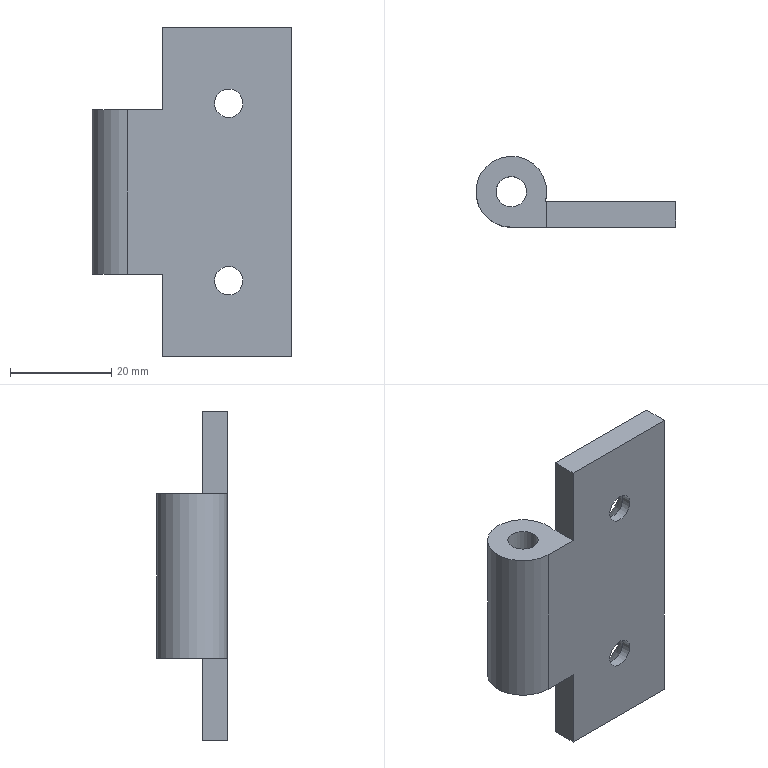Part | NX | 1 solid | 15 faces | box 39.5 x 14 x 65 mm | volume 12285 mm3 | plane 9 | cylinder 4 | cone 2 | commonest cylinder face diameters 5.6 x2 6 x1 14 x1
STEP:
#1=CARTESIAN_POINT('',(7.,0.,0.));
#2=VERTEX_POINT('',#1);
#3=CARTESIAN_POINT('',(7.,5.,0.));
#4=VERTEX_POINT('',#3);
#5=CARTESIAN_POINT('',(7.,-65.,0.));
#6=DIRECTION('',(0.,1.,0.));
#7=VECTOR('',#6,1000.);
#8=LINE('',#5,#7);
#9=EDGE_CURVE('',#2,#4,#8,.T.);
#10=ORIENTED_EDGE('',*,*,#9,.F.);
#11=CARTESIAN_POINT('',(32.5,0.,0.));
#12=VERTEX_POINT('',#11);
#13=CARTESIAN_POINT('',(0.,0.,0.));
#14=DIRECTION('',(1.,0.,0.));
#15=VECTOR('',#14,1000.);
#16=LINE('',#13,#15);
#17=EDGE_CURVE('',#2,#12,#16,.T.);
#18=ORIENTED_EDGE('',*,*,#17,.T.);
#19=CARTESIAN_POINT('',(32.5,5.,0.));
#20=VERTEX_POINT('',#19);
#21=CARTESIAN_POINT('',(32.5,0.,0.));
#22=DIRECTION('',(0.,1.,0.));
#23=VECTOR('',#22,1000.);
#24=LINE('',#21,#23);
#25=EDGE_CURVE('',#12,#20,#24,.T.);
#26=ORIENTED_EDGE('',*,*,#25,.T.);
#27=CARTESIAN_POINT('',(32.5,5.,0.));
#28=DIRECTION('',(-1.,0.,0.));
#29=VECTOR('',#28,1000.);
#30=LINE('',#27,#29);
#31=EDGE_CURVE('',#20,#4,#30,.T.);
#32=ORIENTED_EDGE('',*,*,#31,.T.);
#33=EDGE_LOOP('',(#10,#18,#26,#32));
#34=FACE_BOUND('',#33,.T.);
#35=CARTESIAN_POINT('',(0.,7.,0.));
#36=DIRECTION('',(0.,0.,1.));
#37=DIRECTION('',(1.,0.,0.));
#38=AXIS2_PLACEMENT_3D('',#35,#36,#37);
#39=PLANE('',#38);
#40=ADVANCED_FACE('',(#34),#39,.T.);
#41=CARTESIAN_POINT('',(7.,0.,-65.));
#42=VERTEX_POINT('',#41);
#43=CARTESIAN_POINT('',(32.5,0.,-65.));
#44=VERTEX_POINT('',#43);
#45=CARTESIAN_POINT('',(0.,0.,-65.));
#46=DIRECTION('',(1.,0.,0.));
#47=VECTOR('',#46,1000.);
#48=LINE('',#45,#47);
#49=EDGE_CURVE('',#42,#44,#48,.T.);
#50=ORIENTED_EDGE('',*,*,#49,.F.);
#51=CARTESIAN_POINT('',(7.,5.,-65.));
#52=VERTEX_POINT('',#51);
#53=CARTESIAN_POINT('',(7.,-65.,-65.));
#54=DIRECTION('',(0.,1.,0.));
#55=VECTOR('',#54,1000.);
#56=LINE('',#53,#55);
#57=EDGE_CURVE('',#42,#52,#56,.T.);
#58=ORIENTED_EDGE('',*,*,#57,.T.);
#59=CARTESIAN_POINT('',(32.5,5.,-65.));
#60=VERTEX_POINT('',#59);
#61=CARTESIAN_POINT('',(32.5,5.,-65.));
#62=DIRECTION('',(-1.,0.,0.));
#63=VECTOR('',#62,1000.);
#64=LINE('',#61,#63);
#65=EDGE_CURVE('',#60,#52,#64,.T.);
#66=ORIENTED_EDGE('',*,*,#65,.F.);
#67=CARTESIAN_POINT('',(32.5,0.,-65.));
#68=DIRECTION('',(0.,1.,0.));
#69=VECTOR('',#68,1000.);
#70=LINE('',#67,#69);
#71=EDGE_CURVE('',#44,#60,#70,.T.);
#72=ORIENTED_EDGE('',*,*,#71,.F.);
#73=EDGE_LOOP('',(#50,#58,#66,#72));
#74=FACE_BOUND('',#73,.T.);
#75=CARTESIAN_POINT('',(0.,7.,-65.));
#76=DIRECTION('',(0.,0.,1.));
#77=DIRECTION('',(1.,0.,0.));
#78=AXIS2_PLACEMENT_3D('',#75,#76,#77);
#79=PLANE('',#78);
#80=ADVANCED_FACE('',(#74),#79,.F.);
#81=CARTESIAN_POINT('',(0.,0.,-16.25));
#82=VERTEX_POINT('',#81);
#83=CARTESIAN_POINT('',(6.708,5.,-16.25));
#84=VERTEX_POINT('',#83);
#85=CARTESIAN_POINT('',(0.,7.,-16.25));
#86=DIRECTION('',(0.,0.,-1.));
#87=DIRECTION('',(-1.,0.,0.));
#88=AXIS2_PLACEMENT_3D('',#85,#86,#87);
#89=CIRCLE('',#88,7.);
#90=EDGE_CURVE('',#82,#84,#89,.T.);
#91=ORIENTED_EDGE('',*,*,#90,.T.);
#92=CARTESIAN_POINT('',(6.708,5.,-48.75));
#93=VERTEX_POINT('',#92);
#94=CARTESIAN_POINT('',(6.708,5.,0.));
#95=DIRECTION('',(0.,0.,-1.));
#96=VECTOR('',#95,1000.);
#97=LINE('',#94,#96);
#98=EDGE_CURVE('',#84,#93,#97,.T.);
#99=ORIENTED_EDGE('',*,*,#98,.T.);
#100=CARTESIAN_POINT('',(0.,0.,-48.75));
#101=VERTEX_POINT('',#100);
#102=CARTESIAN_POINT('',(0.,7.,-48.75));
#103=DIRECTION('',(0.,0.,1.));
#104=DIRECTION('',(1.,0.,0.));
#105=AXIS2_PLACEMENT_3D('',#102,#103,#104);
#106=CIRCLE('',#105,7.);
#107=EDGE_CURVE('',#93,#101,#106,.T.);
#108=ORIENTED_EDGE('',*,*,#107,.T.);
#109=CARTESIAN_POINT('',(0.,0.,0.));
#110=DIRECTION('',(0.,0.,-1.));
#111=VECTOR('',#110,1000.);
#112=LINE('',#109,#111);
#113=EDGE_CURVE('',#82,#101,#112,.T.);
#114=ORIENTED_EDGE('',*,*,#113,.F.);
#115=EDGE_LOOP('',(#91,#99,#108,#114));
#116=FACE_BOUND('',#115,.T.);
#117=CARTESIAN_POINT('',(0.,7.,0.));
#118=DIRECTION('',(0.,0.,-1.));
#119=DIRECTION('',(-1.,0.,0.));
#120=AXIS2_PLACEMENT_3D('',#117,#118,#119);
#121=CYLINDRICAL_SURFACE('',#120,7.);
#122=ADVANCED_FACE('',(#116),#121,.T.);
#123=CARTESIAN_POINT('',(20.,0.,-47.2));
#124=VERTEX_POINT('',#123);
#125=CARTESIAN_POINT('',(20.,0.,-50.));
#126=DIRECTION('',(0.,1.,0.));
#127=DIRECTION('',(0.,0.,1.));
#128=AXIS2_PLACEMENT_3D('',#125,#126,#127);
#129=CIRCLE('',#128,2.8);
#130=EDGE_CURVE('',#124,#124,#129,.T.);
#131=ORIENTED_EDGE('',*,*,#130,.T.);
#132=EDGE_LOOP('',(#131));
#133=FACE_BOUND('',#132,.T.);
#134=CARTESIAN_POINT('',(20.,0.,-12.2));
#135=VERTEX_POINT('',#134);
#136=CARTESIAN_POINT('',(20.,0.,-15.));
#137=DIRECTION('',(0.,1.,0.));
#138=DIRECTION('',(0.,0.,1.));
#139=AXIS2_PLACEMENT_3D('',#136,#137,#138);
#140=CIRCLE('',#139,2.8);
#141=EDGE_CURVE('',#135,#135,#140,.T.);
#142=ORIENTED_EDGE('',*,*,#141,.T.);
#143=EDGE_LOOP('',(#142));
#144=FACE_BOUND('',#143,.T.);
#145=CARTESIAN_POINT('',(7.,0.,-48.75));
#146=VERTEX_POINT('',#145);
#147=CARTESIAN_POINT('',(0.,0.,-48.75));
#148=DIRECTION('',(1.,0.,0.));
#149=VECTOR('',#148,1000.);
#150=LINE('',#147,#149);
#151=EDGE_CURVE('',#101,#146,#150,.T.);
#152=ORIENTED_EDGE('',*,*,#151,.T.);
#153=CARTESIAN_POINT('',(7.,0.,0.));
#154=DIRECTION('',(0.,0.,-1.));
#155=VECTOR('',#154,1000.);
#156=LINE('',#153,#155);
#157=EDGE_CURVE('',#146,#42,#156,.T.);
#158=ORIENTED_EDGE('',*,*,#157,.T.);
#159=ORIENTED_EDGE('',*,*,#49,.T.);
#160=CARTESIAN_POINT('',(32.5,0.,0.));
#161=DIRECTION('',(0.,0.,-1.));
#162=VECTOR('',#161,1000.);
#163=LINE('',#160,#162);
#164=EDGE_CURVE('',#12,#44,#163,.T.);
#165=ORIENTED_EDGE('',*,*,#164,.F.);
#166=ORIENTED_EDGE('',*,*,#17,.F.);
#167=CARTESIAN_POINT('',(7.,0.,-16.25));
#168=VERTEX_POINT('',#167);
#169=CARTESIAN_POINT('',(7.,0.,0.));
#170=DIRECTION('',(0.,0.,-1.));
#171=VECTOR('',#170,1000.);
#172=LINE('',#169,#171);
#173=EDGE_CURVE('',#2,#168,#172,.T.);
#174=ORIENTED_EDGE('',*,*,#173,.T.);
#175=CARTESIAN_POINT('',(0.,0.,-16.25));
#176=DIRECTION('',(-1.,0.,0.));
#177=VECTOR('',#176,1000.);
#178=LINE('',#175,#177);
#179=EDGE_CURVE('',#168,#82,#178,.T.);
#180=ORIENTED_EDGE('',*,*,#179,.T.);
#181=ORIENTED_EDGE('',*,*,#113,.T.);
#182=EDGE_LOOP('',(#152,#158,#159,#165,#166,#174,#180,#181));
#183=FACE_BOUND('',#182,.T.);
#184=CARTESIAN_POINT('',(0.,0.,0.));
#185=DIRECTION('',(0.,1.,0.));
#186=DIRECTION('',(0.,0.,1.));
#187=AXIS2_PLACEMENT_3D('',#184,#185,#186);
#188=PLANE('',#187);
#189=ADVANCED_FACE('',(#133,#144,#183),#188,.F.);
#190=ORIENTED_EDGE('',*,*,#71,.T.);
#191=CARTESIAN_POINT('',(32.5,5.,0.));
#192=DIRECTION('',(0.,0.,-1.));
#193=VECTOR('',#192,1000.);
#194=LINE('',#191,#193);
#195=EDGE_CURVE('',#20,#60,#194,.T.);
#196=ORIENTED_EDGE('',*,*,#195,.F.);
#197=ORIENTED_EDGE('',*,*,#25,.F.);
#198=ORIENTED_EDGE('',*,*,#164,.T.);
#199=EDGE_LOOP('',(#190,#196,#197,#198));
#200=FACE_BOUND('',#199,.T.);
#201=CARTESIAN_POINT('',(32.5,0.,0.));
#202=DIRECTION('',(-1.,0.,0.));
#203=DIRECTION('',(0.,0.,1.));
#204=AXIS2_PLACEMENT_3D('',#201,#202,#203);
#205=PLANE('',#204);
#206=ADVANCED_FACE('',(#200),#205,.F.);
#207=CARTESIAN_POINT('',(20.,5.,-44.7));
#208=VERTEX_POINT('',#207);
#209=CARTESIAN_POINT('',(20.,5.,-50.));
#210=DIRECTION('',(0.,1.,0.));
#211=DIRECTION('',(0.,0.,1.));
#212=AXIS2_PLACEMENT_3D('',#209,#210,#211);
#213=CIRCLE('',#212,5.3);
#214=EDGE_CURVE('',#208,#208,#213,.T.);
#215=ORIENTED_EDGE('',*,*,#214,.F.);
#216=EDGE_LOOP('',(#215));
#217=FACE_BOUND('',#216,.T.);
#218=CARTESIAN_POINT('',(20.,5.,-9.7));
#219=VERTEX_POINT('',#218);
#220=CARTESIAN_POINT('',(20.,5.,-15.));
#221=DIRECTION('',(0.,1.,0.));
#222=DIRECTION('',(0.,0.,1.));
#223=AXIS2_PLACEMENT_3D('',#220,#221,#222);
#224=CIRCLE('',#223,5.3);
#225=EDGE_CURVE('',#219,#219,#224,.T.);
#226=ORIENTED_EDGE('',*,*,#225,.F.);
#227=EDGE_LOOP('',(#226));
#228=FACE_BOUND('',#227,.T.);
#229=ORIENTED_EDGE('',*,*,#65,.T.);
#230=CARTESIAN_POINT('',(7.,5.,-48.75));
#231=VERTEX_POINT('',#230);
#232=CARTESIAN_POINT('',(7.,5.,0.));
#233=DIRECTION('',(0.,0.,1.));
#234=VECTOR('',#233,1000.);
#235=LINE('',#232,#234);
#236=EDGE_CURVE('',#52,#231,#235,.T.);
#237=ORIENTED_EDGE('',*,*,#236,.T.);
#238=CARTESIAN_POINT('',(32.5,5.,-48.75));
#239=DIRECTION('',(-1.,0.,0.));
#240=VECTOR('',#239,1000.);
#241=LINE('',#238,#240);
#242=EDGE_CURVE('',#231,#93,#241,.T.);
#243=ORIENTED_EDGE('',*,*,#242,.T.);
#244=ORIENTED_EDGE('',*,*,#98,.F.);
#245=CARTESIAN_POINT('',(7.,5.,-16.25));
#246=VERTEX_POINT('',#245);
#247=CARTESIAN_POINT('',(32.5,5.,-16.25));
#248=DIRECTION('',(1.,0.,0.));
#249=VECTOR('',#248,1000.);
#250=LINE('',#247,#249);
#251=EDGE_CURVE('',#84,#246,#250,.T.);
#252=ORIENTED_EDGE('',*,*,#251,.T.);
#253=CARTESIAN_POINT('',(7.,5.,0.));
#254=DIRECTION('',(0.,0.,1.));
#255=VECTOR('',#254,1000.);
#256=LINE('',#253,#255);
#257=EDGE_CURVE('',#246,#4,#256,.T.);
#258=ORIENTED_EDGE('',*,*,#257,.T.);
#259=ORIENTED_EDGE('',*,*,#31,.F.);
#260=ORIENTED_EDGE('',*,*,#195,.T.);
#261=EDGE_LOOP('',(#229,#237,#243,#244,#252,#258,#259,#260));
#262=FACE_BOUND('',#261,.T.);
#263=CARTESIAN_POINT('',(32.5,5.,0.));
#264=DIRECTION('',(0.,-1.,0.));
#265=DIRECTION('',(0.,0.,-1.));
#266=AXIS2_PLACEMENT_3D('',#263,#264,#265);
#267=PLANE('',#266);
#268=ADVANCED_FACE('',(#217,#228,#262),#267,.F.);
#269=CARTESIAN_POINT('',(-3.,7.,-16.25));
#270=VERTEX_POINT('',#269);
#271=CARTESIAN_POINT('',(0.,7.,-16.25));
#272=DIRECTION('',(0.,0.,-1.));
#273=DIRECTION('',(-1.,0.,0.));
#274=AXIS2_PLACEMENT_3D('',#271,#272,#273);
#275=CIRCLE('',#274,3.);
#276=EDGE_CURVE('',#270,#270,#275,.T.);
#277=ORIENTED_EDGE('',*,*,#276,.T.);
#278=EDGE_LOOP('',(#277));
#279=FACE_BOUND('',#278,.T.);
#280=CARTESIAN_POINT('',(7.,-65.,-16.25));
#281=DIRECTION('',(0.,1.,0.));
#282=VECTOR('',#281,1000.);
#283=LINE('',#280,#282);
#284=EDGE_CURVE('',#168,#246,#283,.T.);
#285=ORIENTED_EDGE('',*,*,#284,.T.);
#286=ORIENTED_EDGE('',*,*,#251,.F.);
#287=ORIENTED_EDGE('',*,*,#90,.F.);
#288=ORIENTED_EDGE('',*,*,#179,.F.);
#289=EDGE_LOOP('',(#285,#286,#287,#288));
#290=FACE_BOUND('',#289,.T.);
#291=CARTESIAN_POINT('',(7.,-65.,-16.25));
#292=DIRECTION('',(0.,0.,-1.));
#293=DIRECTION('',(-1.,0.,0.));
#294=AXIS2_PLACEMENT_3D('',#291,#292,#293);
#295=PLANE('',#294);
#296=ADVANCED_FACE('',(#279,#290),#295,.F.);
#297=ORIENTED_EDGE('',*,*,#9,.T.);
#298=ORIENTED_EDGE('',*,*,#257,.F.);
#299=ORIENTED_EDGE('',*,*,#284,.F.);
#300=ORIENTED_EDGE('',*,*,#173,.F.);
#301=EDGE_LOOP('',(#297,#298,#299,#300));
#302=FACE_BOUND('',#301,.T.);
#303=CARTESIAN_POINT('',(7.,-65.,0.));
#304=DIRECTION('',(1.,0.,0.));
#305=DIRECTION('',(0.,0.,-1.));
#306=AXIS2_PLACEMENT_3D('',#303,#304,#305);
#307=PLANE('',#306);
#308=ADVANCED_FACE('',(#302),#307,.F.);
#309=CARTESIAN_POINT('',(7.,-65.,-48.75));
#310=DIRECTION('',(0.,1.,0.));
#311=VECTOR('',#310,1000.);
#312=LINE('',#309,#311);
#313=EDGE_CURVE('',#146,#231,#312,.T.);
#314=ORIENTED_EDGE('',*,*,#313,.T.);
#315=ORIENTED_EDGE('',*,*,#236,.F.);
#316=ORIENTED_EDGE('',*,*,#57,.F.);
#317=ORIENTED_EDGE('',*,*,#157,.F.);
#318=EDGE_LOOP('',(#314,#315,#316,#317));
#319=FACE_BOUND('',#318,.T.);
#320=CARTESIAN_POINT('',(7.,-65.,-48.75));
#321=DIRECTION('',(1.,0.,0.));
#322=DIRECTION('',(0.,0.,-1.));
#323=AXIS2_PLACEMENT_3D('',#320,#321,#322);
#324=PLANE('',#323);
#325=ADVANCED_FACE('',(#319),#324,.F.);
#326=CARTESIAN_POINT('',(3.,7.,-48.75));
#327=VERTEX_POINT('',#326);
#328=CARTESIAN_POINT('',(0.,7.,-48.75));
#329=DIRECTION('',(0.,0.,1.));
#330=DIRECTION('',(1.,0.,0.));
#331=AXIS2_PLACEMENT_3D('',#328,#329,#330);
#332=CIRCLE('',#331,3.);
#333=EDGE_CURVE('',#327,#327,#332,.T.);
#334=ORIENTED_EDGE('',*,*,#333,.T.);
#335=EDGE_LOOP('',(#334));
#336=FACE_BOUND('',#335,.T.);
#337=ORIENTED_EDGE('',*,*,#107,.F.);
#338=ORIENTED_EDGE('',*,*,#242,.F.);
#339=ORIENTED_EDGE('',*,*,#313,.F.);
#340=ORIENTED_EDGE('',*,*,#151,.F.);
#341=EDGE_LOOP('',(#337,#338,#339,#340));
#342=FACE_BOUND('',#341,.T.);
#343=CARTESIAN_POINT('',(-7.,-65.,-48.75));
#344=DIRECTION('',(0.,0.,1.));
#345=DIRECTION('',(1.,0.,0.));
#346=AXIS2_PLACEMENT_3D('',#343,#344,#345);
#347=PLANE('',#346);
#348=ADVANCED_FACE('',(#336,#342),#347,.F.);
#349=ORIENTED_EDGE('',*,*,#333,.F.);
#350=EDGE_LOOP('',(#349));
#351=FACE_BOUND('',#350,.T.);
#352=ORIENTED_EDGE('',*,*,#276,.F.);
#353=EDGE_LOOP('',(#352));
#354=FACE_BOUND('',#353,.T.);
#355=CARTESIAN_POINT('',(0.,7.,0.));
#356=DIRECTION('',(0.,0.,-1.));
#357=DIRECTION('',(-1.,0.,0.));
#358=AXIS2_PLACEMENT_3D('',#355,#356,#357);
#359=CYLINDRICAL_SURFACE('',#358,3.);
#360=ADVANCED_FACE('',(#351,#354),#359,.F.);
#361=ORIENTED_EDGE('',*,*,#141,.F.);
#362=EDGE_LOOP('',(#361));
#363=FACE_BOUND('',#362,.T.);
#364=CARTESIAN_POINT('',(20.,1.913,-12.2));
#365=VERTEX_POINT('',#364);
#366=CARTESIAN_POINT('',(20.,1.913,-15.));
#367=DIRECTION('',(0.,1.,0.));
#368=DIRECTION('',(0.,0.,1.));
#369=AXIS2_PLACEMENT_3D('',#366,#367,#368);
#370=CIRCLE('',#369,2.8);
#371=EDGE_CURVE('',#365,#365,#370,.T.);
#372=ORIENTED_EDGE('',*,*,#371,.T.);
#373=EDGE_LOOP('',(#372));
#374=FACE_BOUND('',#373,.T.);
#375=CARTESIAN_POINT('',(20.,5.,-15.));
#376=DIRECTION('',(0.,1.,0.));
#377=DIRECTION('',(0.,0.,1.));
#378=AXIS2_PLACEMENT_3D('',#375,#376,#377);
#379=CYLINDRICAL_SURFACE('',#378,2.8);
#380=ADVANCED_FACE('',(#363,#374),#379,.F.);
#381=ORIENTED_EDGE('',*,*,#371,.F.);
#382=EDGE_LOOP('',(#381));
#383=FACE_BOUND('',#382,.T.);
#384=ORIENTED_EDGE('',*,*,#225,.T.);
#385=EDGE_LOOP('',(#384));
#386=FACE_BOUND('',#385,.T.);
#387=CARTESIAN_POINT('',(20.,5.,-15.));
#388=DIRECTION('',(0.,1.,0.));
#389=DIRECTION('',(0.,0.,1.));
#390=AXIS2_PLACEMENT_3D('',#387,#388,#389);
#391=CONICAL_SURFACE('',#390,5.3,0.6807);
#392=ADVANCED_FACE('',(#383,#386),#391,.F.);
#393=ORIENTED_EDGE('',*,*,#130,.F.);
#394=EDGE_LOOP('',(#393));
#395=FACE_BOUND('',#394,.T.);
#396=CARTESIAN_POINT('',(20.,1.913,-47.2));
#397=VERTEX_POINT('',#396);
#398=CARTESIAN_POINT('',(20.,1.913,-50.));
#399=DIRECTION('',(0.,1.,0.));
#400=DIRECTION('',(0.,0.,1.));
#401=AXIS2_PLACEMENT_3D('',#398,#399,#400);
#402=CIRCLE('',#401,2.8);
#403=EDGE_CURVE('',#397,#397,#402,.T.);
#404=ORIENTED_EDGE('',*,*,#403,.T.);
#405=EDGE_LOOP('',(#404));
#406=FACE_BOUND('',#405,.T.);
#407=CARTESIAN_POINT('',(20.,5.,-50.));
#408=DIRECTION('',(0.,1.,0.));
#409=DIRECTION('',(0.,0.,1.));
#410=AXIS2_PLACEMENT_3D('',#407,#408,#409);
#411=CYLINDRICAL_SURFACE('',#410,2.8);
#412=ADVANCED_FACE('',(#395,#406),#411,.F.);
#413=ORIENTED_EDGE('',*,*,#403,.F.);
#414=EDGE_LOOP('',(#413));
#415=FACE_BOUND('',#414,.T.);
#416=ORIENTED_EDGE('',*,*,#214,.T.);
#417=EDGE_LOOP('',(#416));
#418=FACE_BOUND('',#417,.T.);
#419=CARTESIAN_POINT('',(20.,5.,-50.));
#420=DIRECTION('',(0.,1.,0.));
#421=DIRECTION('',(0.,0.,1.));
#422=AXIS2_PLACEMENT_3D('',#419,#420,#421);
#423=CONICAL_SURFACE('',#422,5.3,0.6807);
#424=ADVANCED_FACE('',(#415,#418),#423,.F.);
#425=CLOSED_SHELL('',(#40,#80,#122,#189,#206,#268,#296,#308,#325,#348,#360,#380,#392,#412,#424));
#426=MANIFOLD_SOLID_BREP('',#425);
#427=(LENGTH_UNIT()NAMED_UNIT(*)SI_UNIT(.MILLI.,.METRE.));
#428=UNCERTAINTY_MEASURE_WITH_UNIT(LENGTH_MEASURE(0.00001),#427,'','');
#429=(NAMED_UNIT(*)PLANE_ANGLE_UNIT()SI_UNIT($,.RADIAN.));
#430=(NAMED_UNIT(*)SI_UNIT($,.STERADIAN.)SOLID_ANGLE_UNIT());
#431=(GEOMETRIC_REPRESENTATION_CONTEXT(3)GLOBAL_UNCERTAINTY_ASSIGNED_CONTEXT((#428))GLOBAL_UNIT_ASSIGNED_CONTEXT((#427,#429,#430))REPRESENTATION_CONTEXT('',''));
#432=ADVANCED_BREP_SHAPE_REPRESENTATION('',(#426),#431);